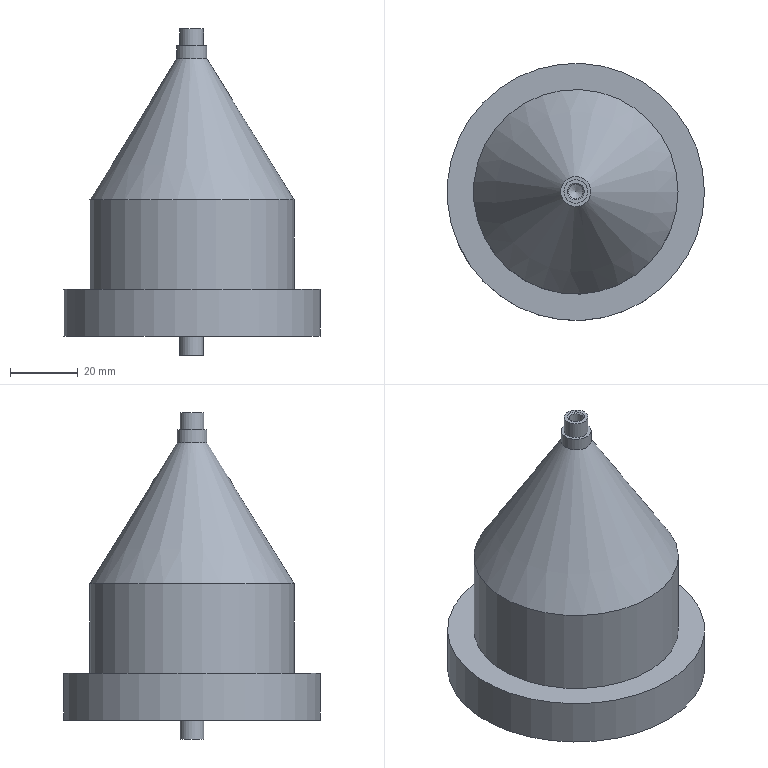Part | STEP file | Radial combiner inner cavity | 3 solids | 47 faces | box 76 x 76 x 96.43 mm | volume 185605 mm3 | cone 21 | cylinder 17 | plane 9 | commonest cylinder face diameters 1.6 x8 2.05 x2 7 x2 4.2 x1 5.7 x1 8.9 x1